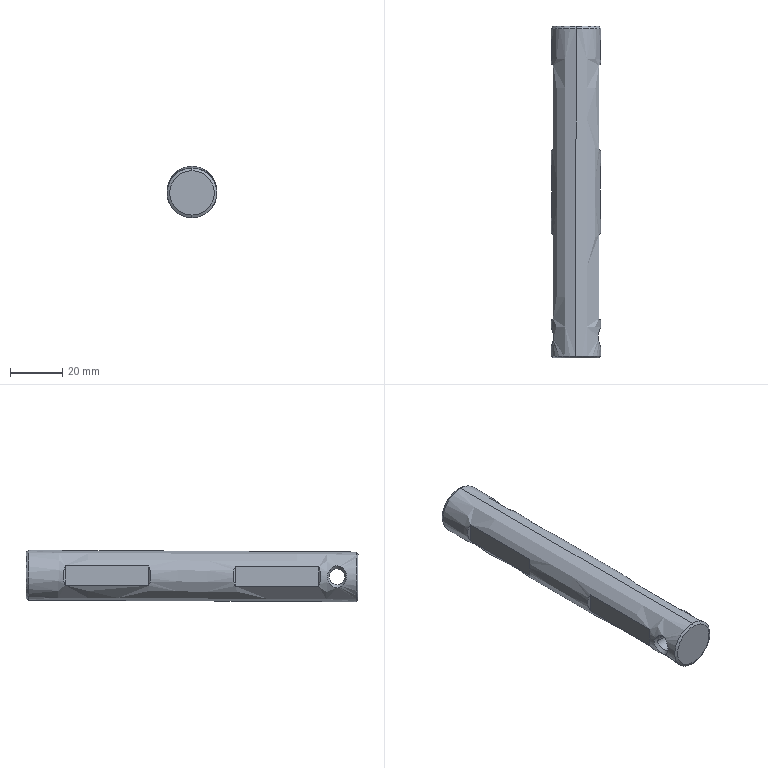Part | NX | features BREP 1 | 1 solid | 26 faces | box 19.05 x 127.075 x 19.691 mm | volume 35013 mm3 | plane 14 | cone 6 | spline 4 | cylinder 2 | commonest cylinder face diameters 6.1 x2